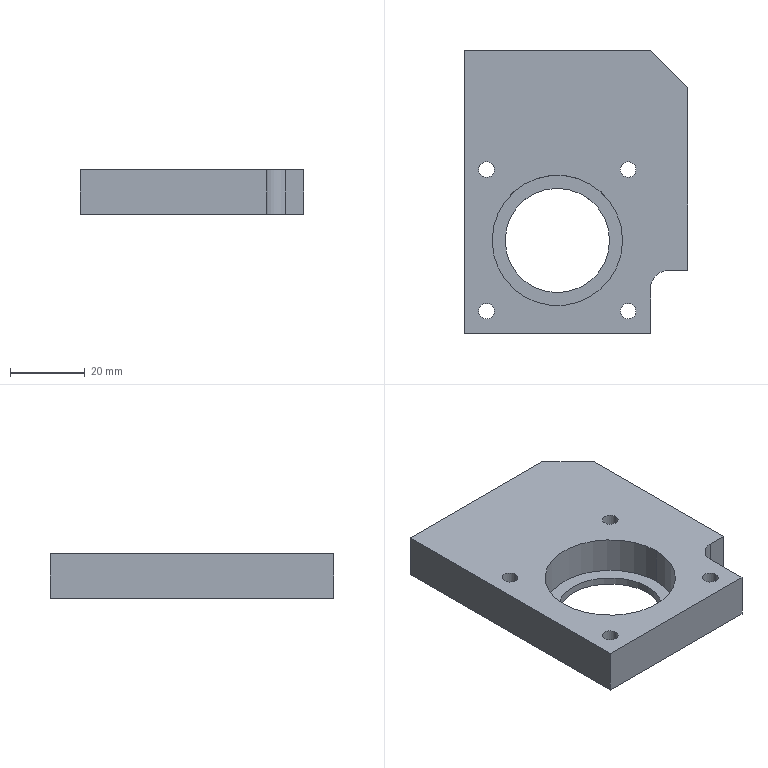Part | SolidWorks | features HoleWzd 2, MoveFace 2, MirrorStock 1 | 1 solid | 43 faces | box 60 x 76 x 12 mm | volume 39739 mm3 | cylinder 23 | cone 10 | plane 10 | commonest cylinder face diameters 4.2 x18 28 x2 35 x2 10 x1
STEP:
#1=CARTESIAN_POINT('',(17.6,22.,2.1));
#2=VERTEX_POINT('',#1);
#3=CARTESIAN_POINT('',(17.6,22.,-2.1));
#4=VERTEX_POINT('',#3);
#5=CARTESIAN_POINT('',(17.6,22.,0.));
#6=DIRECTION('',(-1.,0.,0.));
#7=DIRECTION('',(0.,0.,1.));
#8=AXIS2_PLACEMENT_3D('',#5,#6,#7);
#9=CIRCLE('',#8,2.1);
#10=EDGE_CURVE('',#2,#4,#9,.T.);
#11=ORIENTED_EDGE('',*,*,#10,.T.);
#12=CARTESIAN_POINT('',(30.,22.,-2.1));
#13=VERTEX_POINT('',#12);
#14=CARTESIAN_POINT('',(30.,22.,-2.1));
#15=DIRECTION('',(1.,0.,0.));
#16=VECTOR('',#15,1000.);
#17=LINE('',#14,#16);
#18=EDGE_CURVE('',#4,#13,#17,.T.);
#19=ORIENTED_EDGE('',*,*,#18,.T.);
#20=CARTESIAN_POINT('',(30.,22.,2.1));
#21=VERTEX_POINT('',#20);
#22=CARTESIAN_POINT('',(30.,22.,0.));
#23=DIRECTION('',(-1.,0.,0.));
#24=DIRECTION('',(0.,0.,1.));
#25=AXIS2_PLACEMENT_3D('',#22,#23,#24);
#26=CIRCLE('',#25,2.1);
#27=EDGE_CURVE('',#21,#13,#26,.T.);
#28=ORIENTED_EDGE('',*,*,#27,.F.);
#29=CARTESIAN_POINT('',(30.,22.,2.1));
#30=DIRECTION('',(1.,0.,0.));
#31=VECTOR('',#30,1000.);
#32=LINE('',#29,#31);
#33=EDGE_CURVE('',#2,#21,#32,.T.);
#34=ORIENTED_EDGE('',*,*,#33,.F.);
#35=EDGE_LOOP('',(#11,#19,#28,#34));
#36=FACE_OUTER_BOUND('',#35,.T.);
#37=CARTESIAN_POINT('',(30.,22.,0.));
#38=DIRECTION('',(1.,0.,0.));
#39=DIRECTION('',(0.,0.,1.));
#40=AXIS2_PLACEMENT_3D('',#37,#38,#39);
#41=CYLINDRICAL_SURFACE('',#40,2.1);
#42=ADVANCED_FACE('',(#36),#41,.F.);
#43=CARTESIAN_POINT('',(16.338,22.,0.));
#44=VERTEX_POINT('',#43);
#45=CARTESIAN_POINT('',(17.6,22.,2.1));
#46=DIRECTION('',(0.515,0.,0.8572));
#47=VECTOR('',#46,1000.);
#48=LINE('',#45,#47);
#49=EDGE_CURVE('',#44,#2,#48,.T.);
#50=ORIENTED_EDGE('',*,*,#49,.F.);
#51=CARTESIAN_POINT('',(17.6,22.,-2.1));
#52=DIRECTION('',(0.515,0.,-0.8572));
#53=VECTOR('',#52,1000.);
#54=LINE('',#51,#53);
#55=EDGE_CURVE('',#44,#4,#54,.T.);
#56=ORIENTED_EDGE('',*,*,#55,.T.);
#57=ORIENTED_EDGE('',*,*,#10,.F.);
#58=EDGE_LOOP('',(#50,#56,#57));
#59=FACE_OUTER_BOUND('',#58,.T.);
#60=CARTESIAN_POINT('',(17.6,22.,0.));
#61=DIRECTION('',(1.,0.,0.));
#62=DIRECTION('',(0.,0.,1.));
#63=AXIS2_PLACEMENT_3D('',#60,#61,#62);
#64=CONICAL_SURFACE('',#63,2.1,1.03);
#65=ADVANCED_FACE('',(#59),#64,.F.);
#66=CARTESIAN_POINT('',(17.6,-6.,2.1));
#67=VERTEX_POINT('',#66);
#68=CARTESIAN_POINT('',(17.6,-6.,-2.1));
#69=VERTEX_POINT('',#68);
#70=CARTESIAN_POINT('',(17.6,-6.,0.));
#71=DIRECTION('',(-1.,0.,0.));
#72=DIRECTION('',(0.,0.,1.));
#73=AXIS2_PLACEMENT_3D('',#70,#71,#72);
#74=CIRCLE('',#73,2.1);
#75=EDGE_CURVE('',#67,#69,#74,.T.);
#76=ORIENTED_EDGE('',*,*,#75,.T.);
#77=CARTESIAN_POINT('',(30.,-6.,-2.1));
#78=VERTEX_POINT('',#77);
#79=CARTESIAN_POINT('',(30.,-6.,-2.1));
#80=DIRECTION('',(1.,0.,0.));
#81=VECTOR('',#80,1000.);
#82=LINE('',#79,#81);
#83=EDGE_CURVE('',#69,#78,#82,.T.);
#84=ORIENTED_EDGE('',*,*,#83,.T.);
#85=CARTESIAN_POINT('',(30.,-6.,2.1));
#86=VERTEX_POINT('',#85);
#87=CARTESIAN_POINT('',(30.,-6.,0.));
#88=DIRECTION('',(-1.,0.,0.));
#89=DIRECTION('',(0.,0.,1.));
#90=AXIS2_PLACEMENT_3D('',#87,#88,#89);
#91=CIRCLE('',#90,2.1);
#92=EDGE_CURVE('',#86,#78,#91,.T.);
#93=ORIENTED_EDGE('',*,*,#92,.F.);
#94=CARTESIAN_POINT('',(30.,-6.,2.1));
#95=DIRECTION('',(1.,0.,0.));
#96=VECTOR('',#95,1000.);
#97=LINE('',#94,#96);
#98=EDGE_CURVE('',#67,#86,#97,.T.);
#99=ORIENTED_EDGE('',*,*,#98,.F.);
#100=EDGE_LOOP('',(#76,#84,#93,#99));
#101=FACE_OUTER_BOUND('',#100,.T.);
#102=CARTESIAN_POINT('',(30.,-6.,0.));
#103=DIRECTION('',(1.,0.,0.));
#104=DIRECTION('',(0.,0.,1.));
#105=AXIS2_PLACEMENT_3D('',#102,#103,#104);
#106=CYLINDRICAL_SURFACE('',#105,2.1);
#107=ADVANCED_FACE('',(#101),#106,.F.);
#108=CARTESIAN_POINT('',(16.338,-6.,0.));
#109=VERTEX_POINT('',#108);
#110=CARTESIAN_POINT('',(17.6,-6.,2.1));
#111=DIRECTION('',(0.515,0.,0.8572));
#112=VECTOR('',#111,1000.);
#113=LINE('',#110,#112);
#114=EDGE_CURVE('',#109,#67,#113,.T.);
#115=ORIENTED_EDGE('',*,*,#114,.F.);
#116=CARTESIAN_POINT('',(17.6,-6.,-2.1));
#117=DIRECTION('',(0.515,0.,-0.8572));
#118=VECTOR('',#117,1000.);
#119=LINE('',#116,#118);
#120=EDGE_CURVE('',#109,#69,#119,.T.);
#121=ORIENTED_EDGE('',*,*,#120,.T.);
#122=ORIENTED_EDGE('',*,*,#75,.F.);
#123=EDGE_LOOP('',(#115,#121,#122));
#124=FACE_OUTER_BOUND('',#123,.T.);
#125=CARTESIAN_POINT('',(17.6,-6.,0.));
#126=DIRECTION('',(1.,0.,0.));
#127=DIRECTION('',(0.,0.,1.));
#128=AXIS2_PLACEMENT_3D('',#125,#126,#127);
#129=CONICAL_SURFACE('',#128,2.1,1.03);
#130=ADVANCED_FACE('',(#124),#129,.F.);
#131=CARTESIAN_POINT('',(-24.,27.6,-2.1));
#132=VERTEX_POINT('',#131);
#133=CARTESIAN_POINT('',(-24.,27.6,2.1));
#134=VERTEX_POINT('',#133);
#135=CARTESIAN_POINT('',(-24.,27.6,0.));
#136=DIRECTION('',(0.,-1.,0.));
#137=DIRECTION('',(0.,0.,-1.));
#138=AXIS2_PLACEMENT_3D('',#135,#136,#137);
#139=CIRCLE('',#138,2.1);
#140=EDGE_CURVE('',#132,#134,#139,.T.);
#141=ORIENTED_EDGE('',*,*,#140,.T.);
#142=CARTESIAN_POINT('',(-24.,40.,2.1));
#143=VERTEX_POINT('',#142);
#144=CARTESIAN_POINT('',(-24.,40.,2.1));
#145=DIRECTION('',(0.,1.,0.));
#146=VECTOR('',#145,1000.);
#147=LINE('',#144,#146);
#148=EDGE_CURVE('',#134,#143,#147,.T.);
#149=ORIENTED_EDGE('',*,*,#148,.T.);
#150=CARTESIAN_POINT('',(-24.,40.,-2.1));
#151=VERTEX_POINT('',#150);
#152=CARTESIAN_POINT('',(-24.,40.,0.));
#153=DIRECTION('',(0.,-1.,0.));
#154=DIRECTION('',(0.,0.,-1.));
#155=AXIS2_PLACEMENT_3D('',#152,#153,#154);
#156=CIRCLE('',#155,2.1);
#157=EDGE_CURVE('',#151,#143,#156,.T.);
#158=ORIENTED_EDGE('',*,*,#157,.F.);
#159=CARTESIAN_POINT('',(-24.,40.,-2.1));
#160=DIRECTION('',(0.,1.,0.));
#161=VECTOR('',#160,1000.);
#162=LINE('',#159,#161);
#163=EDGE_CURVE('',#132,#151,#162,.T.);
#164=ORIENTED_EDGE('',*,*,#163,.F.);
#165=EDGE_LOOP('',(#141,#149,#158,#164));
#166=FACE_OUTER_BOUND('',#165,.T.);
#167=CARTESIAN_POINT('',(-24.,40.,0.));
#168=DIRECTION('',(0.,1.,0.));
#169=DIRECTION('',(0.,0.,-1.));
#170=AXIS2_PLACEMENT_3D('',#167,#168,#169);
#171=CYLINDRICAL_SURFACE('',#170,2.1);
#172=ADVANCED_FACE('',(#166),#171,.F.);
#173=CARTESIAN_POINT('',(-24.,26.338,0.));
#174=VERTEX_POINT('',#173);
#175=CARTESIAN_POINT('',(-24.,27.6,-2.1));
#176=DIRECTION('',(0.,0.515,-0.8572));
#177=VECTOR('',#176,1000.);
#178=LINE('',#175,#177);
#179=EDGE_CURVE('',#174,#132,#178,.T.);
#180=ORIENTED_EDGE('',*,*,#179,.F.);
#181=CARTESIAN_POINT('',(-24.,27.6,2.1));
#182=DIRECTION('',(0.,0.515,0.8572));
#183=VECTOR('',#182,1000.);
#184=LINE('',#181,#183);
#185=EDGE_CURVE('',#174,#134,#184,.T.);
#186=ORIENTED_EDGE('',*,*,#185,.T.);
#187=ORIENTED_EDGE('',*,*,#140,.F.);
#188=EDGE_LOOP('',(#180,#186,#187));
#189=FACE_OUTER_BOUND('',#188,.T.);
#190=CARTESIAN_POINT('',(-24.,27.6,0.));
#191=DIRECTION('',(0.,1.,0.));
#192=DIRECTION('',(0.,0.,-1.));
#193=AXIS2_PLACEMENT_3D('',#190,#191,#192);
#194=CONICAL_SURFACE('',#193,2.1,1.03);
#195=ADVANCED_FACE('',(#189),#194,.F.);
#196=CARTESIAN_POINT('',(-2.9,27.6,-2.1));
#197=VERTEX_POINT('',#196);
#198=CARTESIAN_POINT('',(-2.9,27.6,2.1));
#199=VERTEX_POINT('',#198);
#200=CARTESIAN_POINT('',(-2.9,27.6,0.));
#201=DIRECTION('',(0.,-1.,0.));
#202=DIRECTION('',(0.,0.,-1.));
#203=AXIS2_PLACEMENT_3D('',#200,#201,#202);
#204=CIRCLE('',#203,2.1);
#205=EDGE_CURVE('',#197,#199,#204,.T.);
#206=ORIENTED_EDGE('',*,*,#205,.T.);
#207=CARTESIAN_POINT('',(-2.9,40.,2.1));
#208=VERTEX_POINT('',#207);
#209=CARTESIAN_POINT('',(-2.9,40.,2.1));
#210=DIRECTION('',(0.,1.,0.));
#211=VECTOR('',#210,1000.);
#212=LINE('',#209,#211);
#213=EDGE_CURVE('',#199,#208,#212,.T.);
#214=ORIENTED_EDGE('',*,*,#213,.T.);
#215=CARTESIAN_POINT('',(-2.9,40.,-2.1));
#216=VERTEX_POINT('',#215);
#217=CARTESIAN_POINT('',(-2.9,40.,0.));
#218=DIRECTION('',(0.,-1.,0.));
#219=DIRECTION('',(0.,0.,-1.));
#220=AXIS2_PLACEMENT_3D('',#217,#218,#219);
#221=CIRCLE('',#220,2.1);
#222=EDGE_CURVE('',#216,#208,#221,.T.);
#223=ORIENTED_EDGE('',*,*,#222,.F.);
#224=CARTESIAN_POINT('',(-2.9,40.,-2.1));
#225=DIRECTION('',(0.,1.,0.));
#226=VECTOR('',#225,1000.);
#227=LINE('',#224,#226);
#228=EDGE_CURVE('',#197,#216,#227,.T.);
#229=ORIENTED_EDGE('',*,*,#228,.F.);
#230=EDGE_LOOP('',(#206,#214,#223,#229));
#231=FACE_OUTER_BOUND('',#230,.T.);
#232=CARTESIAN_POINT('',(-2.9,40.,0.));
#233=DIRECTION('',(0.,1.,0.));
#234=DIRECTION('',(0.,0.,-1.));
#235=AXIS2_PLACEMENT_3D('',#232,#233,#234);
#236=CYLINDRICAL_SURFACE('',#235,2.1);
#237=ADVANCED_FACE('',(#231),#236,.F.);
#238=CARTESIAN_POINT('',(-2.9,26.338,0.));
#239=VERTEX_POINT('',#238);
#240=CARTESIAN_POINT('',(-2.9,27.6,-2.1));
#241=DIRECTION('',(0.,0.515,-0.8572));
#242=VECTOR('',#241,1000.);
#243=LINE('',#240,#242);
#244=EDGE_CURVE('',#239,#197,#243,.T.);
#245=ORIENTED_EDGE('',*,*,#244,.F.);
#246=CARTESIAN_POINT('',(-2.9,27.6,2.1));
#247=DIRECTION('',(0.,0.515,0.8572));
#248=VECTOR('',#247,1000.);
#249=LINE('',#246,#248);
#250=EDGE_CURVE('',#239,#199,#249,.T.);
#251=ORIENTED_EDGE('',*,*,#250,.T.);
#252=ORIENTED_EDGE('',*,*,#205,.F.);
#253=EDGE_LOOP('',(#245,#251,#252));
#254=FACE_OUTER_BOUND('',#253,.T.);
#255=CARTESIAN_POINT('',(-2.9,27.6,0.));
#256=DIRECTION('',(0.,1.,0.));
#257=DIRECTION('',(0.,0.,-1.));
#258=AXIS2_PLACEMENT_3D('',#255,#256,#257);
#259=CONICAL_SURFACE('',#258,2.1,1.03);
#260=ADVANCED_FACE('',(#254),#259,.F.);
#261=CARTESIAN_POINT('',(15.,27.6,-2.1));
#262=VERTEX_POINT('',#261);
#263=CARTESIAN_POINT('',(15.,27.6,2.1));
#264=VERTEX_POINT('',#263);
#265=CARTESIAN_POINT('',(15.,27.6,0.));
#266=DIRECTION('',(0.,-1.,0.));
#267=DIRECTION('',(0.,0.,-1.));
#268=AXIS2_PLACEMENT_3D('',#265,#266,#267);
#269=CIRCLE('',#268,2.1);
#270=EDGE_CURVE('',#262,#264,#269,.T.);
#271=ORIENTED_EDGE('',*,*,#270,.T.);
#272=CARTESIAN_POINT('',(15.,40.,2.1));
#273=VERTEX_POINT('',#272);
#274=CARTESIAN_POINT('',(15.,40.,2.1));
#275=DIRECTION('',(0.,1.,0.));
#276=VECTOR('',#275,1000.);
#277=LINE('',#274,#276);
#278=EDGE_CURVE('',#264,#273,#277,.T.);
#279=ORIENTED_EDGE('',*,*,#278,.T.);
#280=CARTESIAN_POINT('',(15.,40.,-2.1));
#281=VERTEX_POINT('',#280);
#282=CARTESIAN_POINT('',(15.,40.,0.));
#283=DIRECTION('',(0.,-1.,0.));
#284=DIRECTION('',(0.,0.,-1.));
#285=AXIS2_PLACEMENT_3D('',#282,#283,#284);
#286=CIRCLE('',#285,2.1);
#287=EDGE_CURVE('',#281,#273,#286,.T.);
#288=ORIENTED_EDGE('',*,*,#287,.F.);
#289=CARTESIAN_POINT('',(15.,40.,-2.1));
#290=DIRECTION('',(0.,1.,0.));
#291=VECTOR('',#290,1000.);
#292=LINE('',#289,#291);
#293=EDGE_CURVE('',#262,#281,#292,.T.);
#294=ORIENTED_EDGE('',*,*,#293,.F.);
#295=EDGE_LOOP('',(#271,#279,#288,#294));
#296=FACE_OUTER_BOUND('',#295,.T.);
#297=CARTESIAN_POINT('',(15.,40.,0.));
#298=DIRECTION('',(0.,1.,0.));
#299=DIRECTION('',(0.,0.,-1.));
#300=AXIS2_PLACEMENT_3D('',#297,#298,#299);
#301=CYLINDRICAL_SURFACE('',#300,2.1);
#302=ADVANCED_FACE('',(#296),#301,.F.);
#303=CARTESIAN_POINT('',(15.,26.338,0.));
#304=VERTEX_POINT('',#303);
#305=CARTESIAN_POINT('',(15.,27.6,-2.1));
#306=DIRECTION('',(0.,0.515,-0.8572));
#307=VECTOR('',#306,1000.);
#308=LINE('',#305,#307);
#309=EDGE_CURVE('',#304,#262,#308,.T.);
#310=ORIENTED_EDGE('',*,*,#309,.F.);
#311=CARTESIAN_POINT('',(15.,27.6,2.1));
#312=DIRECTION('',(0.,0.515,0.8572));
#313=VECTOR('',#312,1000.);
#314=LINE('',#311,#313);
#315=EDGE_CURVE('',#304,#264,#314,.T.);
#316=ORIENTED_EDGE('',*,*,#315,.T.);
#317=ORIENTED_EDGE('',*,*,#270,.F.);
#318=EDGE_LOOP('',(#310,#316,#317));
#319=FACE_OUTER_BOUND('',#318,.T.);
#320=CARTESIAN_POINT('',(15.,27.6,0.));
#321=DIRECTION('',(0.,1.,0.));
#322=DIRECTION('',(0.,0.,-1.));
#323=AXIS2_PLACEMENT_3D('',#320,#321,#322);
#324=CONICAL_SURFACE('',#323,2.1,1.03);
#325=ADVANCED_FACE('',(#319),#324,.F.);
#326=CARTESIAN_POINT('',(11.9,8.,-6.));
#327=VERTEX_POINT('',#326);
#328=CARTESIAN_POINT('',(16.1,8.,-6.));
#329=VERTEX_POINT('',#328);
#330=CARTESIAN_POINT('',(14.,8.,-6.));
#331=DIRECTION('',(0.,0.,-1.));
#332=DIRECTION('',(-1.,0.,0.));
#333=AXIS2_PLACEMENT_3D('',#330,#331,#332);
#334=CIRCLE('',#333,2.1);
#335=EDGE_CURVE('',#327,#329,#334,.T.);
#336=ORIENTED_EDGE('',*,*,#335,.T.);
#337=CARTESIAN_POINT('',(16.1,8.,6.));
#338=VERTEX_POINT('',#337);
#339=CARTESIAN_POINT('',(16.1,8.,6.));
#340=DIRECTION('',(0.,0.,1.));
#341=VECTOR('',#340,1000.);
#342=LINE('',#339,#341);
#343=EDGE_CURVE('',#329,#338,#342,.T.);
#344=ORIENTED_EDGE('',*,*,#343,.T.);
#345=CARTESIAN_POINT('',(11.9,8.,6.));
#346=VERTEX_POINT('',#345);
#347=CARTESIAN_POINT('',(14.,8.,6.));
#348=DIRECTION('',(0.,0.,-1.));
#349=DIRECTION('',(-1.,0.,0.));
#350=AXIS2_PLACEMENT_3D('',#347,#348,#349);
#351=CIRCLE('',#350,2.1);
#352=EDGE_CURVE('',#346,#338,#351,.T.);
#353=ORIENTED_EDGE('',*,*,#352,.F.);
#354=CARTESIAN_POINT('',(11.9,8.,6.));
#355=DIRECTION('',(0.,0.,1.));
#356=VECTOR('',#355,1000.);
#357=LINE('',#354,#356);
#358=EDGE_CURVE('',#327,#346,#357,.T.);
#359=ORIENTED_EDGE('',*,*,#358,.F.);
#360=EDGE_LOOP('',(#336,#344,#353,#359));
#361=FACE_OUTER_BOUND('',#360,.T.);
#362=CARTESIAN_POINT('',(14.,8.,6.));
#363=DIRECTION('',(0.,0.,1.));
#364=DIRECTION('',(-1.,0.,0.));
#365=AXIS2_PLACEMENT_3D('',#362,#363,#364);
#366=CYLINDRICAL_SURFACE('',#365,2.1);
#367=ADVANCED_FACE('',(#361),#366,.F.);
#368=CARTESIAN_POINT('',(11.9,-30.,-6.));
#369=VERTEX_POINT('',#368);
#370=CARTESIAN_POINT('',(16.1,-30.,-6.));
#371=VERTEX_POINT('',#370);
#372=CARTESIAN_POINT('',(14.,-30.,-6.));
#373=DIRECTION('',(0.,0.,-1.));
#374=DIRECTION('',(-1.,0.,0.));
#375=AXIS2_PLACEMENT_3D('',#372,#373,#374);
#376=CIRCLE('',#375,2.1);
#377=EDGE_CURVE('',#369,#371,#376,.T.);
#378=ORIENTED_EDGE('',*,*,#377,.T.);
#379=CARTESIAN_POINT('',(16.1,-30.,6.));
#380=VERTEX_POINT('',#379);
#381=CARTESIAN_POINT('',(16.1,-30.,6.));
#382=DIRECTION('',(0.,0.,1.));
#383=VECTOR('',#382,1000.);
#384=LINE('',#381,#383);
#385=EDGE_CURVE('',#371,#380,#384,.T.);
#386=ORIENTED_EDGE('',*,*,#385,.T.);
#387=CARTESIAN_POINT('',(11.9,-30.,6.));
#388=VERTEX_POINT('',#387);
#389=CARTESIAN_POINT('',(14.,-30.,6.));
#390=DIRECTION('',(0.,0.,-1.));
#391=DIRECTION('',(-1.,0.,0.));
#392=AXIS2_PLACEMENT_3D('',#389,#390,#391);
#393=CIRCLE('',#392,2.1);
#394=EDGE_CURVE('',#388,#380,#393,.T.);
#395=ORIENTED_EDGE('',*,*,#394,.F.);
#396=CARTESIAN_POINT('',(11.9,-30.,6.));
#397=DIRECTION('',(0.,0.,1.));
#398=VECTOR('',#397,1000.);
#399=LINE('',#396,#398);
#400=EDGE_CURVE('',#369,#388,#399,.T.);
#401=ORIENTED_EDGE('',*,*,#400,.F.);
#402=EDGE_LOOP('',(#378,#386,#395,#401));
#403=FACE_OUTER_BOUND('',#402,.T.);
#404=CARTESIAN_POINT('',(14.,-30.,6.));
#405=DIRECTION('',(0.,0.,1.));
#406=DIRECTION('',(-1.,0.,0.));
#407=AXIS2_PLACEMENT_3D('',#404,#405,#406);
#408=CYLINDRICAL_SURFACE('',#407,2.1);
#409=ADVANCED_FACE('',(#403),#408,.F.);
#410=CARTESIAN_POINT('',(-26.1,-30.,-6.));
#411=VERTEX_POINT('',#410);
#412=CARTESIAN_POINT('',(-21.9,-30.,-6.));
#413=VERTEX_POINT('',#412);
#414=CARTESIAN_POINT('',(-24.,-30.,-6.));
#415=DIRECTION('',(0.,0.,-1.));
#416=DIRECTION('',(-1.,0.,0.));
#417=AXIS2_PLACEMENT_3D('',#414,#415,#416);
#418=CIRCLE('',#417,2.1);
#419=EDGE_CURVE('',#411,#413,#418,.T.);
#420=ORIENTED_EDGE('',*,*,#419,.T.);
#421=CARTESIAN_POINT('',(-21.9,-30.,6.));
#422=VERTEX_POINT('',#421);
#423=CARTESIAN_POINT('',(-21.9,-30.,6.));
#424=DIRECTION('',(0.,0.,1.));
#425=VECTOR('',#424,1000.);
#426=LINE('',#423,#425);
#427=EDGE_CURVE('',#413,#422,#426,.T.);
#428=ORIENTED_EDGE('',*,*,#427,.T.);
#429=CARTESIAN_POINT('',(-26.1,-30.,6.));
#430=VERTEX_POINT('',#429);
#431=CARTESIAN_POINT('',(-24.,-30.,6.));
#432=DIRECTION('',(0.,0.,-1.));
#433=DIRECTION('',(-1.,0.,0.));
#434=AXIS2_PLACEMENT_3D('',#431,#432,#433);
#435=CIRCLE('',#434,2.1);
#436=EDGE_CURVE('',#430,#422,#435,.T.);
#437=ORIENTED_EDGE('',*,*,#436,.F.);
#438=CARTESIAN_POINT('',(-26.1,-30.,6.));
#439=DIRECTION('',(0.,0.,1.));
#440=VECTOR('',#439,1000.);
#441=LINE('',#438,#440);
#442=EDGE_CURVE('',#411,#430,#441,.T.);
#443=ORIENTED_EDGE('',*,*,#442,.F.);
#444=EDGE_LOOP('',(#420,#428,#437,#443));
#445=FACE_OUTER_BOUND('',#444,.T.);
#446=CARTESIAN_POINT('',(-24.,-30.,6.));
#447=DIRECTION('',(0.,0.,1.));
#448=DIRECTION('',(-1.,0.,0.));
#449=AXIS2_PLACEMENT_3D('',#446,#447,#448);
#450=CYLINDRICAL_SURFACE('',#449,2.1);
#451=ADVANCED_FACE('',(#445),#450,.F.);
#452=CARTESIAN_POINT('',(-26.1,8.,-6.));
#453=VERTEX_POINT('',#452);
#454=CARTESIAN_POINT('',(-21.9,8.,-6.));
#455=VERTEX_POINT('',#454);
#456=CARTESIAN_POINT('',(-24.,8.,-6.));
#457=DIRECTION('',(0.,0.,-1.));
#458=DIRECTION('',(-1.,0.,0.));
#459=AXIS2_PLACEMENT_3D('',#456,#457,#458);
#460=CIRCLE('',#459,2.1);
#461=EDGE_CURVE('',#453,#455,#460,.T.);
#462=ORIENTED_EDGE('',*,*,#461,.T.);
#463=CARTESIAN_POINT('',(-21.9,8.,6.));
#464=VERTEX_POINT('',#463);
#465=CARTESIAN_POINT('',(-21.9,8.,6.));
#466=DIRECTION('',(0.,0.,1.));
#467=VECTOR('',#466,1000.);
#468=LINE('',#465,#467);
#469=EDGE_CURVE('',#455,#464,#468,.T.);
#470=ORIENTED_EDGE('',*,*,#469,.T.);
#471=CARTESIAN_POINT('',(-26.1,8.,6.));
#472=VERTEX_POINT('',#471);
#473=CARTESIAN_POINT('',(-24.,8.,6.));
#474=DIRECTION('',(0.,0.,-1.));
#475=DIRECTION('',(-1.,0.,0.));
#476=AXIS2_PLACEMENT_3D('',#473,#474,#475);
#477=CIRCLE('',#476,2.1);
#478=EDGE_CURVE('',#472,#464,#477,.T.);
#479=ORIENTED_EDGE('',*,*,#478,.F.);
#480=CARTESIAN_POINT('',(-26.1,8.,6.));
#481=DIRECTION('',(0.,0.,1.));
#482=VECTOR('',#481,1000.);
#483=LINE('',#480,#482);
#484=EDGE_CURVE('',#453,#472,#483,.T.);
#485=ORIENTED_EDGE('',*,*,#484,.F.);
#486=EDGE_LOOP('',(#462,#470,#479,#485));
#487=FACE_OUTER_BOUND('',#486,.T.);
#488=CARTESIAN_POINT('',(-24.,8.,6.));
#489=DIRECTION('',(0.,0.,1.));
#490=DIRECTION('',(-1.,0.,0.));
#491=AXIS2_PLACEMENT_3D('',#488,#489,#490);
#492=CYLINDRICAL_SURFACE('',#491,2.1);
#493=ADVANCED_FACE('',(#487),#492,.F.);
#494=CARTESIAN_POINT('',(-19.,-11.,-6.));
#495=VERTEX_POINT('',#494);
#496=CARTESIAN_POINT('',(9.,-11.,-6.));
#497=VERTEX_POINT('',#496);
#498=CARTESIAN_POINT('',(-5.,-11.,-6.));
#499=DIRECTION('',(0.,0.,-1.));
#500=DIRECTION('',(-1.,0.,0.));
#501=AXIS2_PLACEMENT_3D('',#498,#499,#500);
#502=CIRCLE('',#501,14.);
#503=EDGE_CURVE('',#495,#497,#502,.T.);
#504=ORIENTED_EDGE('',*,*,#503,.T.);
#505=CARTESIAN_POINT('',(9.,-11.,-4.));
#506=VERTEX_POINT('',#505);
#507=CARTESIAN_POINT('',(9.,-11.,-6.));
#508=DIRECTION('',(0.,0.,1.));
#509=VECTOR('',#508,1000.);
#510=LINE('',#507,#509);
#511=EDGE_CURVE('',#497,#506,#510,.T.);
#512=ORIENTED_EDGE('',*,*,#511,.T.);
#513=CARTESIAN_POINT('',(-19.,-11.,-4.));
#514=VERTEX_POINT('',#513);
#515=CARTESIAN_POINT('',(-5.,-11.,-4.));
#516=DIRECTION('',(0.,0.,-1.));
#517=DIRECTION('',(-1.,0.,0.));
#518=AXIS2_PLACEMENT_3D('',#515,#516,#517);
#519=CIRCLE('',#518,14.);
#520=EDGE_CURVE('',#514,#506,#519,.T.);
#521=ORIENTED_EDGE('',*,*,#520,.F.);
#522=CARTESIAN_POINT('',(-19.,-11.,-6.));
#523=DIRECTION('',(0.,0.,1.));
#524=VECTOR('',#523,1000.);
#525=LINE('',#522,#524);
#526=EDGE_CURVE('',#495,#514,#525,.T.);
#527=ORIENTED_EDGE('',*,*,#526,.F.);
#528=EDGE_LOOP('',(#504,#512,#521,#527));
#529=FACE_OUTER_BOUND('',#528,.T.);
#530=CARTESIAN_POINT('',(-5.,-11.,-6.));
#531=DIRECTION('',(0.,0.,1.));
#532=DIRECTION('',(-1.,0.,0.));
#533=AXIS2_PLACEMENT_3D('',#530,#531,#532);
#534=CYLINDRICAL_SURFACE('',#533,14.);
#535=ADVANCED_FACE('',(#529),#534,.F.);
#536=CARTESIAN_POINT('',(12.5,-11.,-4.));
#537=VERTEX_POINT('',#536);
#538=CARTESIAN_POINT('',(-22.5,-11.,-4.));
#539=VERTEX_POINT('',#538);
#540=CARTESIAN_POINT('',(-5.,-11.,-4.));
#541=DIRECTION('',(0.,0.,1.));
#542=DIRECTION('',(1.,0.,0.));
#543=AXIS2_PLACEMENT_3D('',#540,#541,#542);
#544=CIRCLE('',#543,17.5);
#545=EDGE_CURVE('',#537,#539,#544,.T.);
#546=ORIENTED_EDGE('',*,*,#545,.F.);
#547=CARTESIAN_POINT('',(12.5,-11.,6.));
#548=VERTEX_POINT('',#547);
#549=CARTESIAN_POINT('',(12.5,-11.,-4.));
#550=DIRECTION('',(0.,0.,1.));
#551=VECTOR('',#550,1000.);
#552=LINE('',#549,#551);
#553=EDGE_CURVE('',#537,#548,#552,.T.);
#554=ORIENTED_EDGE('',*,*,#553,.T.);
#555=CARTESIAN_POINT('',(-22.5,-11.,6.));
#556=VERTEX_POINT('',#555);
#557=CARTESIAN_POINT('',(-5.,-11.,6.));
#558=DIRECTION('',(0.,0.,1.));
#559=DIRECTION('',(1.,0.,0.));
#560=AXIS2_PLACEMENT_3D('',#557,#558,#559);
#561=CIRCLE('',#560,17.5);
#562=EDGE_CURVE('',#548,#556,#561,.T.);
#563=ORIENTED_EDGE('',*,*,#562,.T.);
#564=CARTESIAN_POINT('',(-22.5,-11.,-4.));
#565=DIRECTION('',(0.,0.,1.));
#566=VECTOR('',#565,1000.);
#567=LINE('',#564,#566);
#568=EDGE_CURVE('',#539,#556,#567,.T.);
#569=ORIENTED_EDGE('',*,*,#568,.F.);
#570=EDGE_LOOP('',(#546,#554,#563,#569));
#571=FACE_OUTER_BOUND('',#570,.T.);
#572=CARTESIAN_POINT('',(-5.,-11.,-4.));
#573=DIRECTION('',(0.,0.,1.));
#574=DIRECTION('',(-1.,0.,0.));
#575=AXIS2_PLACEMENT_3D('',#572,#573,#574);
#576=CYLINDRICAL_SURFACE('',#575,17.5);
#577=ADVANCED_FACE('',(#571),#576,.F.);
#578=ORIENTED_EDGE('',*,*,#27,.T.);
#579=CARTESIAN_POINT('',(30.,22.,0.));
#580=DIRECTION('',(-1.,0.,0.));
#581=DIRECTION('',(0.,0.,1.));
#582=AXIS2_PLACEMENT_3D('',#579,#580,#581);
#583=CIRCLE('',#582,2.1);
#584=EDGE_CURVE('',#13,#21,#583,.T.);
#585=ORIENTED_EDGE('',*,*,#584,.T.);
#586=EDGE_LOOP('',(#578,#585));
#587=FACE_BOUND('',#586,.T.);
#588=ORIENTED_EDGE('',*,*,#92,.T.);
#589=CARTESIAN_POINT('',(30.,-6.,0.));
#590=DIRECTION('',(-1.,0.,0.));
#591=DIRECTION('',(0.,0.,1.));
#592=AXIS2_PLACEMENT_3D('',#589,#590,#591);
#593=CIRCLE('',#592,2.1);
#594=EDGE_CURVE('',#78,#86,#593,.T.);
#595=ORIENTED_EDGE('',*,*,#594,.T.);
#596=EDGE_LOOP('',(#588,#595));
#597=FACE_BOUND('',#596,.T.);
#598=CARTESIAN_POINT('',(30.,-19.,6.));
#599=VERTEX_POINT('',#598);
#600=CARTESIAN_POINT('',(30.,30.,6.));
#601=VERTEX_POINT('',#600);
#602=CARTESIAN_POINT('',(30.,-41.,6.));
#603=DIRECTION('',(0.,1.,0.));
#604=VECTOR('',#603,1000.);
#605=LINE('',#602,#604);
#606=EDGE_CURVE('',#599,#601,#605,.T.);
#607=ORIENTED_EDGE('',*,*,#606,.F.);
#608=CARTESIAN_POINT('',(30.,-19.,-6.));
#609=VERTEX_POINT('',#608);
#610=CARTESIAN_POINT('',(30.,-19.,6.));
#611=DIRECTION('',(0.,0.,-1.));
#612=VECTOR('',#611,1000.);
#613=LINE('',#610,#612);
#614=EDGE_CURVE('',#599,#609,#613,.T.);
#615=ORIENTED_EDGE('',*,*,#614,.T.);
#616=CARTESIAN_POINT('',(30.,30.,-6.));
#617=VERTEX_POINT('',#616);
#618=CARTESIAN_POINT('',(30.,-41.,-6.));
#619=DIRECTION('',(0.,1.,0.));
#620=VECTOR('',#619,1000.);
#621=LINE('',#618,#620);
#622=EDGE_CURVE('',#609,#617,#621,.T.);
#623=ORIENTED_EDGE('',*,*,#622,.T.);
#624=CARTESIAN_POINT('',(30.,30.,-6.));
#625=DIRECTION('',(0.,0.,-1.));
#626=VECTOR('',#625,1000.);
#627=LINE('',#624,#626);
#628=EDGE_CURVE('',#601,#617,#627,.T.);
#629=ORIENTED_EDGE('',*,*,#628,.F.);
#630=EDGE_LOOP('',(#607,#615,#623,#629));
#631=FACE_OUTER_BOUND('',#630,.T.);
#632=CARTESIAN_POINT('',(30.,-41.,-6.));
#633=DIRECTION('',(-1.,0.,0.));
#634=DIRECTION('',(0.,0.,-1.));
#635=AXIS2_PLACEMENT_3D('',#632,#633,#634);
#636=PLANE('',#635);
#637=ADVANCED_FACE('',(#587,#597,#631),#636,.F.);
#638=ORIENTED_EDGE('',*,*,#157,.T.);
#639=CARTESIAN_POINT('',(-24.,40.,0.));
#640=DIRECTION('',(0.,-1.,0.));
#641=DIRECTION('',(0.,0.,-1.));
#642=AXIS2_PLACEMENT_3D('',#639,#640,#641);
#643=CIRCLE('',#642,2.1);
#644=EDGE_CURVE('',#143,#151,#643,.T.);
#645=ORIENTED_EDGE('',*,*,#644,.T.);
#646=EDGE_LOOP('',(#638,#645));
#647=FACE_BOUND('',#646,.T.);
#648=ORIENTED_EDGE('',*,*,#222,.T.);
#649=CARTESIAN_POINT('',(-2.9,40.,0.));
#650=DIRECTION('',(0.,-1.,0.));
#651=DIRECTION('',(0.,0.,-1.));
#652=AXIS2_PLACEMENT_3D('',#649,#650,#651);
#653=CIRCLE('',#652,2.1);
#654=EDGE_CURVE('',#208,#216,#653,.T.);
#655=ORIENTED_EDGE('',*,*,#654,.T.);
#656=EDGE_LOOP('',(#648,#655));
#657=FACE_BOUND('',#656,.T.);
#658=ORIENTED_EDGE('',*,*,#287,.T.);
#659=CARTESIAN_POINT('',(15.,40.,0.));
#660=DIRECTION('',(0.,-1.,0.));
#661=DIRECTION('',(0.,0.,-1.));
#662=AXIS2_PLACEMENT_3D('',#659,#660,#661);
#663=CIRCLE('',#662,2.1);
#664=EDGE_CURVE('',#273,#281,#663,.T.);
#665=ORIENTED_EDGE('',*,*,#664,.T.);
#666=EDGE_LOOP('',(#658,#665));
#667=FACE_BOUND('',#666,.T.);
#668=CARTESIAN_POINT('',(20.,40.,-6.));
#669=VERTEX_POINT('',#668);
#670=CARTESIAN_POINT('',(-30.,40.,-6.));
#671=VERTEX_POINT('',#670);
#672=CARTESIAN_POINT('',(-30.,40.,-6.));
#673=DIRECTION('',(-1.,0.,0.));
#674=VECTOR('',#673,1000.);
#675=LINE('',#672,#674);
#676=EDGE_CURVE('',#669,#671,#675,.T.);
#677=ORIENTED_EDGE('',*,*,#676,.T.);
#678=CARTESIAN_POINT('',(-30.,40.,6.));
#679=VERTEX_POINT('',#678);
#680=CARTESIAN_POINT('',(-30.,40.,-6.));
#681=DIRECTION('',(0.,0.,1.));
#682=VECTOR('',#681,1000.);
#683=LINE('',#680,#682);
#684=EDGE_CURVE('',#671,#679,#683,.T.);
#685=ORIENTED_EDGE('',*,*,#684,.T.);
#686=CARTESIAN_POINT('',(20.,40.,6.));
#687=VERTEX_POINT('',#686);
#688=CARTESIAN_POINT('',(-30.,40.,6.));
#689=DIRECTION('',(-1.,0.,0.));
#690=VECTOR('',#689,1000.);
#691=LINE('',#688,#690);
#692=EDGE_CURVE('',#687,#679,#691,.T.);
#693=ORIENTED_EDGE('',*,*,#692,.F.);
#694=CARTESIAN_POINT('',(20.,40.,-6.));
#695=DIRECTION('',(0.,0.,1.));
#696=VECTOR('',#695,1000.);
#697=LINE('',#694,#696);
#698=EDGE_CURVE('',#669,#687,#697,.T.);
#699=ORIENTED_EDGE('',*,*,#698,.F.);
#700=EDGE_LOOP('',(#677,#685,#693,#699));
#701=FACE_OUTER_BOUND('',#700,.T.);
#702=CARTESIAN_POINT('',(-30.,40.,-6.));
#703=DIRECTION('',(0.,-1.,0.));
#704=DIRECTION('',(0.,0.,1.));
#705=AXIS2_PLACEMENT_3D('',#702,#703,#704);
#706=PLANE('',#705);
#707=ADVANCED_FACE('',(#647,#657,#667,#701),#706,.F.);
#708=CARTESIAN_POINT('',(-30.,-36.,6.));
#709=VERTEX_POINT('',#708);
#710=CARTESIAN_POINT('',(-30.,-41.,6.));
#711=DIRECTION('',(0.,-1.,0.));
#712=VECTOR('',#711,1000.);
#713=LINE('',#710,#712);
#714=EDGE_CURVE('',#679,#709,#713,.T.);
#715=ORIENTED_EDGE('',*,*,#714,.F.);
#716=ORIENTED_EDGE('',*,*,#684,.F.);
#717=CARTESIAN_POINT('',(-30.,-36.,-6.));
#718=VERTEX_POINT('',#717);
#719=CARTESIAN_POINT('',(-30.,-41.,-6.));
#720=DIRECTION('',(0.,-1.,0.));
#721=VECTOR('',#720,1000.);
#722=LINE('',#719,#721);
#723=EDGE_CURVE('',#671,#718,#722,.T.);
#724=ORIENTED_EDGE('',*,*,#723,.T.);
#725=CARTESIAN_POINT('',(-30.,-36.,-6.));
#726=DIRECTION('',(0.,0.,1.));
#727=VECTOR('',#726,1000.);
#728=LINE('',#725,#727);
#729=EDGE_CURVE('',#718,#709,#728,.T.);
#730=ORIENTED_EDGE('',*,*,#729,.T.);
#731=EDGE_LOOP('',(#715,#716,#724,#730));
#732=FACE_OUTER_BOUND('',#731,.T.);
#733=CARTESIAN_POINT('',(-30.,-41.,-6.));
#734=DIRECTION('',(1.,0.,0.));
#735=DIRECTION('',(0.,0.,1.));
#736=AXIS2_PLACEMENT_3D('',#733,#734,#735);
#737=PLANE('',#736);
#738=ADVANCED_FACE('',(#732),#737,.F.);
#739=CARTESIAN_POINT('',(20.,-36.,6.));
#740=VERTEX_POINT('',#739);
#741=CARTESIAN_POINT('',(-30.,-36.,6.));
#742=DIRECTION('',(1.,0.,0.));
#743=VECTOR('',#742,1000.);
#744=LINE('',#741,#743);
#745=EDGE_CURVE('',#709,#740,#744,.T.);
#746=ORIENTED_EDGE('',*,*,#745,.F.);
#747=ORIENTED_EDGE('',*,*,#729,.F.);
#748=CARTESIAN_POINT('',(20.,-36.,-6.));
#749=VERTEX_POINT('',#748);
#750=CARTESIAN_POINT('',(-30.,-36.,-6.));
#751=DIRECTION('',(1.,0.,0.));
#752=VECTOR('',#751,1000.);
#753=LINE('',#750,#752);
#754=EDGE_CURVE('',#718,#749,#753,.T.);
#755=ORIENTED_EDGE('',*,*,#754,.T.);
#756=CARTESIAN_POINT('',(20.,-36.,6.));
#757=DIRECTION('',(0.,0.,-1.));
#758=VECTOR('',#757,1000.);
#759=LINE('',#756,#758);
#760=EDGE_CURVE('',#740,#749,#759,.T.);
#761=ORIENTED_EDGE('',*,*,#760,.F.);
#762=EDGE_LOOP('',(#746,#747,#755,#761));
#763=FACE_OUTER_BOUND('',#762,.T.);
#764=CARTESIAN_POINT('',(-30.,-36.,-6.));
#765=DIRECTION('',(0.,1.,0.));
#766=DIRECTION('',(0.,0.,-1.));
#767=AXIS2_PLACEMENT_3D('',#764,#765,#766);
#768=PLANE('',#767);
#769=ADVANCED_FACE('',(#763),#768,.F.);
#770=ORIENTED_EDGE('',*,*,#335,.F.);
#771=CARTESIAN_POINT('',(14.,8.,-6.));
#772=DIRECTION('',(0.,0.,-1.));
#773=DIRECTION('',(-1.,0.,0.));
#774=AXIS2_PLACEMENT_3D('',#771,#772,#773);
#775=CIRCLE('',#774,2.1);
#776=EDGE_CURVE('',#329,#327,#775,.T.);
#777=ORIENTED_EDGE('',*,*,#776,.F.);
#778=EDGE_LOOP('',(#770,#777));
#779=FACE_BOUND('',#778,.T.);
#780=ORIENTED_EDGE('',*,*,#377,.F.);
#781=CARTESIAN_POINT('',(14.,-30.,-6.));
#782=DIRECTION('',(0.,0.,-1.));
#783=DIRECTION('',(-1.,0.,0.));
#784=AXIS2_PLACEMENT_3D('',#781,#782,#783);
#785=CIRCLE('',#784,2.1);
#786=EDGE_CURVE('',#371,#369,#785,.T.);
#787=ORIENTED_EDGE('',*,*,#786,.F.);
#788=EDGE_LOOP('',(#780,#787));
#789=FACE_BOUND('',#788,.T.);
#790=ORIENTED_EDGE('',*,*,#419,.F.);
#791=CARTESIAN_POINT('',(-24.,-30.,-6.));
#792=DIRECTION('',(0.,0.,-1.));
#793=DIRECTION('',(-1.,0.,0.));
#794=AXIS2_PLACEMENT_3D('',#791,#792,#793);
#795=CIRCLE('',#794,2.1);
#796=EDGE_CURVE('',#413,#411,#795,.T.);
#797=ORIENTED_EDGE('',*,*,#796,.F.);
#798=EDGE_LOOP('',(#790,#797));
#799=FACE_BOUND('',#798,.T.);
#800=ORIENTED_EDGE('',*,*,#461,.F.);
#801=CARTESIAN_POINT('',(-24.,8.,-6.));
#802=DIRECTION('',(0.,0.,-1.));
#803=DIRECTION('',(-1.,0.,0.));
#804=AXIS2_PLACEMENT_3D('',#801,#802,#803);
#805=CIRCLE('',#804,2.1);
#806=EDGE_CURVE('',#455,#453,#805,.T.);
#807=ORIENTED_EDGE('',*,*,#806,.F.);
#808=EDGE_LOOP('',(#800,#807));
#809=FACE_BOUND('',#808,.T.);
#810=ORIENTED_EDGE('',*,*,#503,.F.);
#811=CARTESIAN_POINT('',(-5.,-11.,-6.));
#812=DIRECTION('',(0.,0.,-1.));
#813=DIRECTION('',(-1.,0.,0.));
#814=AXIS2_PLACEMENT_3D('',#811,#812,#813);
#815=CIRCLE('',#814,14.);
#816=EDGE_CURVE('',#497,#495,#815,.T.);
#817=ORIENTED_EDGE('',*,*,#816,.F.);
#818=EDGE_LOOP('',(#810,#817));
#819=FACE_BOUND('',#818,.T.);
#820=ORIENTED_EDGE('',*,*,#622,.F.);
#821=CARTESIAN_POINT('',(25.,-19.,-6.));
#822=VERTEX_POINT('',#821);
#823=CARTESIAN_POINT('',(20.,-19.,-6.));
#824=DIRECTION('',(-1.,0.,0.));
#825=VECTOR('',#824,1000.);
#826=LINE('',#823,#825);
#827=EDGE_CURVE('',#609,#822,#826,.T.);
#828=ORIENTED_EDGE('',*,*,#827,.T.);
#829=CARTESIAN_POINT('',(20.,-24.,-6.));
#830=VERTEX_POINT('',#829);
#831=CARTESIAN_POINT('',(25.,-24.,-6.));
#832=DIRECTION('',(0.,0.,-1.));
#833=DIRECTION('',(-1.,0.,0.));
#834=AXIS2_PLACEMENT_3D('',#831,#832,#833);
#835=CIRCLE('',#834,5.);
#836=EDGE_CURVE('',#830,#822,#835,.T.);
#837=ORIENTED_EDGE('',*,*,#836,.F.);
#838=CARTESIAN_POINT('',(20.,-41.,-6.));
#839=DIRECTION('',(0.,-1.,0.));
#840=VECTOR('',#839,1000.);
#841=LINE('',#838,#840);
#842=EDGE_CURVE('',#830,#749,#841,.T.);
#843=ORIENTED_EDGE('',*,*,#842,.T.);
#844=ORIENTED_EDGE('',*,*,#754,.F.);
#845=ORIENTED_EDGE('',*,*,#723,.F.);
#846=ORIENTED_EDGE('',*,*,#676,.F.);
#847=CARTESIAN_POINT('',(20.,40.,-6.));
#848=DIRECTION('',(-0.7071,0.7071,0.));
#849=VECTOR('',#848,1000.);
#850=LINE('',#847,#849);
#851=EDGE_CURVE('',#617,#669,#850,.T.);
#852=ORIENTED_EDGE('',*,*,#851,.F.);
#853=EDGE_LOOP('',(#820,#828,#837,#843,#844,#845,#846,#852));
#854=FACE_OUTER_BOUND('',#853,.T.);
#855=CARTESIAN_POINT('',(0.,0.,-6.));
#856=DIRECTION('',(0.,0.,1.));
#857=DIRECTION('',(-1.,0.,0.));
#858=AXIS2_PLACEMENT_3D('',#855,#856,#857);
#859=PLANE('',#858);
#860=ADVANCED_FACE('',(#779,#789,#799,#809,#819,#854),#859,.F.);
#861=ORIENTED_EDGE('',*,*,#352,.T.);
#862=CARTESIAN_POINT('',(14.,8.,6.));
#863=DIRECTION('',(0.,0.,-1.));
#864=DIRECTION('',(-1.,0.,0.));
#865=AXIS2_PLACEMENT_3D('',#862,#863,#864);
#866=CIRCLE('',#865,2.1);
#867=EDGE_CURVE('',#338,#346,#866,.T.);
#868=ORIENTED_EDGE('',*,*,#867,.T.);
#869=EDGE_LOOP('',(#861,#868));
#870=FACE_BOUND('',#869,.T.);
#871=ORIENTED_EDGE('',*,*,#394,.T.);
#872=CARTESIAN_POINT('',(14.,-30.,6.));
#873=DIRECTION('',(0.,0.,-1.));
#874=DIRECTION('',(-1.,0.,0.));
#875=AXIS2_PLACEMENT_3D('',#872,#873,#874);
#876=CIRCLE('',#875,2.1);
#877=EDGE_CURVE('',#380,#388,#876,.T.);
#878=ORIENTED_EDGE('',*,*,#877,.T.);
#879=EDGE_LOOP('',(#871,#878));
#880=FACE_BOUND('',#879,.T.);
#881=ORIENTED_EDGE('',*,*,#436,.T.);
#882=CARTESIAN_POINT('',(-24.,-30.,6.));
#883=DIRECTION('',(0.,0.,-1.));
#884=DIRECTION('',(-1.,0.,0.));
#885=AXIS2_PLACEMENT_3D('',#882,#883,#884);
#886=CIRCLE('',#885,2.1);
#887=EDGE_CURVE('',#422,#430,#886,.T.);
#888=ORIENTED_EDGE('',*,*,#887,.T.);
#889=EDGE_LOOP('',(#881,#888));
#890=FACE_BOUND('',#889,.T.);
#891=ORIENTED_EDGE('',*,*,#478,.T.);
#892=CARTESIAN_POINT('',(-24.,8.,6.));
#893=DIRECTION('',(0.,0.,-1.));
#894=DIRECTION('',(-1.,0.,0.));
#895=AXIS2_PLACEMENT_3D('',#892,#893,#894);
#896=CIRCLE('',#895,2.1);
#897=EDGE_CURVE('',#464,#472,#896,.T.);
#898=ORIENTED_EDGE('',*,*,#897,.T.);
#899=EDGE_LOOP('',(#891,#898));
#900=FACE_BOUND('',#899,.T.);
#901=ORIENTED_EDGE('',*,*,#692,.T.);
#902=ORIENTED_EDGE('',*,*,#714,.T.);
#903=ORIENTED_EDGE('',*,*,#745,.T.);
#904=CARTESIAN_POINT('',(20.,-24.,6.));
#905=VERTEX_POINT('',#904);
#906=CARTESIAN_POINT('',(20.,-41.,6.));
#907=DIRECTION('',(0.,-1.,0.));
#908=VECTOR('',#907,1000.);
#909=LINE('',#906,#908);
#910=EDGE_CURVE('',#905,#740,#909,.T.);
#911=ORIENTED_EDGE('',*,*,#910,.F.);
#912=CARTESIAN_POINT('',(25.,-19.,6.));
#913=VERTEX_POINT('',#912);
#914=CARTESIAN_POINT('',(25.,-24.,6.));
#915=DIRECTION('',(0.,0.,1.));
#916=DIRECTION('',(-1.,0.,0.));
#917=AXIS2_PLACEMENT_3D('',#914,#915,#916);
#918=CIRCLE('',#917,5.);
#919=EDGE_CURVE('',#913,#905,#918,.T.);
#920=ORIENTED_EDGE('',*,*,#919,.F.);
#921=CARTESIAN_POINT('',(20.,-19.,6.));
#922=DIRECTION('',(-1.,0.,0.));
#923=VECTOR('',#922,1000.);
#924=LINE('',#921,#923);
#925=EDGE_CURVE('',#599,#913,#924,.T.);
#926=ORIENTED_EDGE('',*,*,#925,.F.);
#927=ORIENTED_EDGE('',*,*,#606,.T.);
#928=CARTESIAN_POINT('',(30.,30.,6.));
#929=DIRECTION('',(0.7071,-0.7071,0.));
#930=VECTOR('',#929,1000.);
#931=LINE('',#928,#930);
#932=EDGE_CURVE('',#687,#601,#931,.T.);
#933=ORIENTED_EDGE('',*,*,#932,.F.);
#934=EDGE_LOOP('',(#901,#902,#903,#911,#920,#926,#927,#933));
#935=FACE_OUTER_BOUND('',#934,.T.);
#936=CARTESIAN_POINT('',(-5.,-11.,6.));
#937=DIRECTION('',(0.,0.,1.));
#938=DIRECTION('',(1.,0.,0.));
#939=AXIS2_PLACEMENT_3D('',#936,#937,#938);
#940=CIRCLE('',#939,17.5);
#941=EDGE_CURVE('',#556,#548,#940,.T.);
#942=ORIENTED_EDGE('',*,*,#941,.F.);
#943=ORIENTED_EDGE('',*,*,#562,.F.);
#944=EDGE_LOOP('',(#942,#943));
#945=FACE_BOUND('',#944,.T.);
#946=CARTESIAN_POINT('',(0.,0.,6.));
#947=DIRECTION('',(0.,0.,1.));
#948=DIRECTION('',(-1.,0.,0.));
#949=AXIS2_PLACEMENT_3D('',#946,#947,#948);
#950=PLANE('',#949);
#951=ADVANCED_FACE('',(#870,#880,#890,#900,#935,#945),#950,.T.);
#952=ORIENTED_EDGE('',*,*,#553,.F.);
#953=CARTESIAN_POINT('',(-5.,-11.,-4.));
#954=DIRECTION('',(0.,0.,1.));
#955=DIRECTION('',(1.,0.,0.));
#956=AXIS2_PLACEMENT_3D('',#953,#954,#955);
#957=CIRCLE('',#956,17.5);
#958=EDGE_CURVE('',#539,#537,#957,.T.);
#959=ORIENTED_EDGE('',*,*,#958,.F.);
#960=ORIENTED_EDGE('',*,*,#568,.T.);
#961=ORIENTED_EDGE('',*,*,#941,.T.);
#962=EDGE_LOOP('',(#952,#959,#960,#961));
#963=FACE_OUTER_BOUND('',#962,.T.);
#964=CARTESIAN_POINT('',(-5.,-11.,-4.));
#965=DIRECTION('',(0.,0.,1.));
#966=DIRECTION('',(-1.,0.,0.));
#967=AXIS2_PLACEMENT_3D('',#964,#965,#966);
#968=CYLINDRICAL_SURFACE('',#967,17.5);
#969=ADVANCED_FACE('',(#963),#968,.F.);
#970=ORIENTED_EDGE('',*,*,#520,.T.);
#971=CARTESIAN_POINT('',(-5.,-11.,-4.));
#972=DIRECTION('',(0.,0.,-1.));
#973=DIRECTION('',(-1.,0.,0.));
#974=AXIS2_PLACEMENT_3D('',#971,#972,#973);
#975=CIRCLE('',#974,14.);
#976=EDGE_CURVE('',#506,#514,#975,.T.);
#977=ORIENTED_EDGE('',*,*,#976,.T.);
#978=EDGE_LOOP('',(#970,#977));
#979=FACE_BOUND('',#978,.T.);
#980=ORIENTED_EDGE('',*,*,#958,.T.);
#981=ORIENTED_EDGE('',*,*,#545,.T.);
#982=EDGE_LOOP('',(#980,#981));
#983=FACE_OUTER_BOUND('',#982,.T.);
#984=CARTESIAN_POINT('',(-5.,-11.,-4.));
#985=DIRECTION('',(0.,0.,-1.));
#986=DIRECTION('',(1.,0.,0.));
#987=AXIS2_PLACEMENT_3D('',#984,#985,#986);
#988=PLANE('',#987);
#989=ADVANCED_FACE('',(#979,#983),#988,.F.);
#990=ORIENTED_EDGE('',*,*,#511,.F.);
#991=ORIENTED_EDGE('',*,*,#816,.T.);
#992=ORIENTED_EDGE('',*,*,#526,.T.);
#993=ORIENTED_EDGE('',*,*,#976,.F.);
#994=EDGE_LOOP('',(#990,#991,#992,#993));
#995=FACE_OUTER_BOUND('',#994,.T.);
#996=CARTESIAN_POINT('',(-5.,-11.,-6.));
#997=DIRECTION('',(0.,0.,1.));
#998=DIRECTION('',(-1.,0.,0.));
#999=AXIS2_PLACEMENT_3D('',#996,#997,#998);
#1000=CYLINDRICAL_SURFACE('',#999,14.);
#1001=ADVANCED_FACE('',(#995),#1000,.F.);
#1002=ORIENTED_EDGE('',*,*,#910,.T.);
#1003=ORIENTED_EDGE('',*,*,#760,.T.);
#1004=ORIENTED_EDGE('',*,*,#842,.F.);
#1005=CARTESIAN_POINT('',(20.,-24.,-6.));
#1006=DIRECTION('',(0.,0.,-1.));
#1007=VECTOR('',#1006,1000.);
#1008=LINE('',#1005,#1007);
#1009=EDGE_CURVE('',#905,#830,#1008,.T.);
#1010=ORIENTED_EDGE('',*,*,#1009,.F.);
#1011=EDGE_LOOP('',(#1002,#1003,#1004,#1010));
#1012=FACE_OUTER_BOUND('',#1011,.T.);
#1013=CARTESIAN_POINT('',(20.,-41.,6.));
#1014=DIRECTION('',(-1.,0.,0.));
#1015=DIRECTION('',(0.,0.,-1.));
#1016=AXIS2_PLACEMENT_3D('',#1013,#1014,#1015);
#1017=PLANE('',#1016);
#1018=ADVANCED_FACE('',(#1012),#1017,.F.);
#1019=ORIENTED_EDGE('',*,*,#827,.F.);
#1020=ORIENTED_EDGE('',*,*,#614,.F.);
#1021=ORIENTED_EDGE('',*,*,#925,.T.);
#1022=CARTESIAN_POINT('',(25.,-19.,6.));
#1023=DIRECTION('',(0.,0.,1.));
#1024=VECTOR('',#1023,1000.);
#1025=LINE('',#1022,#1024);
#1026=EDGE_CURVE('',#822,#913,#1025,.T.);
#1027=ORIENTED_EDGE('',*,*,#1026,.F.);
#1028=EDGE_LOOP('',(#1019,#1020,#1021,#1027));
#1029=FACE_OUTER_BOUND('',#1028,.T.);
#1030=CARTESIAN_POINT('',(20.,-19.,6.));
#1031=DIRECTION('',(0.,1.,0.));
#1032=DIRECTION('',(0.,0.,-1.));
#1033=AXIS2_PLACEMENT_3D('',#1030,#1031,#1032);
#1034=PLANE('',#1033);
#1035=ADVANCED_FACE('',(#1029),#1034,.F.);
#1036=ORIENTED_EDGE('',*,*,#919,.T.);
#1037=ORIENTED_EDGE('',*,*,#1009,.T.);
#1038=ORIENTED_EDGE('',*,*,#836,.T.);
#1039=ORIENTED_EDGE('',*,*,#1026,.T.);
#1040=EDGE_LOOP('',(#1036,#1037,#1038,#1039));
#1041=FACE_OUTER_BOUND('',#1040,.T.);
#1042=CARTESIAN_POINT('',(25.,-24.,6.));
#1043=DIRECTION('',(0.,0.,1.));
#1044=DIRECTION('',(-1.,0.,0.));
#1045=AXIS2_PLACEMENT_3D('',#1042,#1043,#1044);
#1046=CYLINDRICAL_SURFACE('',#1045,5.);
#1047=ADVANCED_FACE('',(#1041),#1046,.F.);
#1048=ORIENTED_EDGE('',*,*,#469,.F.);
#1049=ORIENTED_EDGE('',*,*,#806,.T.);
#1050=ORIENTED_EDGE('',*,*,#484,.T.);
#1051=ORIENTED_EDGE('',*,*,#897,.F.);
#1052=EDGE_LOOP('',(#1048,#1049,#1050,#1051));
#1053=FACE_OUTER_BOUND('',#1052,.T.);
#1054=CARTESIAN_POINT('',(-24.,8.,6.));
#1055=DIRECTION('',(0.,0.,1.));
#1056=DIRECTION('',(-1.,0.,0.));
#1057=AXIS2_PLACEMENT_3D('',#1054,#1055,#1056);
#1058=CYLINDRICAL_SURFACE('',#1057,2.1);
#1059=ADVANCED_FACE('',(#1053),#1058,.F.);
#1060=ORIENTED_EDGE('',*,*,#427,.F.);
#1061=ORIENTED_EDGE('',*,*,#796,.T.);
#1062=ORIENTED_EDGE('',*,*,#442,.T.);
#1063=ORIENTED_EDGE('',*,*,#887,.F.);
#1064=EDGE_LOOP('',(#1060,#1061,#1062,#1063));
#1065=FACE_OUTER_BOUND('',#1064,.T.);
#1066=CARTESIAN_POINT('',(-24.,-30.,6.));
#1067=DIRECTION('',(0.,0.,1.));
#1068=DIRECTION('',(-1.,0.,0.));
#1069=AXIS2_PLACEMENT_3D('',#1066,#1067,#1068);
#1070=CYLINDRICAL_SURFACE('',#1069,2.1);
#1071=ADVANCED_FACE('',(#1065),#1070,.F.);
#1072=ORIENTED_EDGE('',*,*,#385,.F.);
#1073=ORIENTED_EDGE('',*,*,#786,.T.);
#1074=ORIENTED_EDGE('',*,*,#400,.T.);
#1075=ORIENTED_EDGE('',*,*,#877,.F.);
#1076=EDGE_LOOP('',(#1072,#1073,#1074,#1075));
#1077=FACE_OUTER_BOUND('',#1076,.T.);
#1078=CARTESIAN_POINT('',(14.,-30.,6.));
#1079=DIRECTION('',(0.,0.,1.));
#1080=DIRECTION('',(-1.,0.,0.));
#1081=AXIS2_PLACEMENT_3D('',#1078,#1079,#1080);
#1082=CYLINDRICAL_SURFACE('',#1081,2.1);
#1083=ADVANCED_FACE('',(#1077),#1082,.F.);
#1084=ORIENTED_EDGE('',*,*,#343,.F.);
#1085=ORIENTED_EDGE('',*,*,#776,.T.);
#1086=ORIENTED_EDGE('',*,*,#358,.T.);
#1087=ORIENTED_EDGE('',*,*,#867,.F.);
#1088=EDGE_LOOP('',(#1084,#1085,#1086,#1087));
#1089=FACE_OUTER_BOUND('',#1088,.T.);
#1090=CARTESIAN_POINT('',(14.,8.,6.));
#1091=DIRECTION('',(0.,0.,1.));
#1092=DIRECTION('',(-1.,0.,0.));
#1093=AXIS2_PLACEMENT_3D('',#1090,#1091,#1092);
#1094=CYLINDRICAL_SURFACE('',#1093,2.1);
#1095=ADVANCED_FACE('',(#1089),#1094,.F.);
#1096=ORIENTED_EDGE('',*,*,#851,.T.);
#1097=ORIENTED_EDGE('',*,*,#698,.T.);
#1098=ORIENTED_EDGE('',*,*,#932,.T.);
#1099=ORIENTED_EDGE('',*,*,#628,.T.);
#1100=EDGE_LOOP('',(#1096,#1097,#1098,#1099));
#1101=FACE_OUTER_BOUND('',#1100,.T.);
#1102=CARTESIAN_POINT('',(20.,40.,-6.));
#1103=DIRECTION('',(-0.7071,-0.7071,0.));
#1104=DIRECTION('',(0.,0.,1.));
#1105=AXIS2_PLACEMENT_3D('',#1102,#1103,#1104);
#1106=PLANE('',#1105);
#1107=ADVANCED_FACE('',(#1101),#1106,.F.);
#1108=ORIENTED_EDGE('',*,*,#315,.F.);
#1109=ORIENTED_EDGE('',*,*,#309,.T.);
#1110=CARTESIAN_POINT('',(15.,27.6,0.));
#1111=DIRECTION('',(0.,-1.,0.));
#1112=DIRECTION('',(0.,0.,-1.));
#1113=AXIS2_PLACEMENT_3D('',#1110,#1111,#1112);
#1114=CIRCLE('',#1113,2.1);
#1115=EDGE_CURVE('',#264,#262,#1114,.T.);
#1116=ORIENTED_EDGE('',*,*,#1115,.F.);
#1117=EDGE_LOOP('',(#1108,#1109,#1116));
#1118=FACE_OUTER_BOUND('',#1117,.T.);
#1119=CARTESIAN_POINT('',(15.,27.6,0.));
#1120=DIRECTION('',(0.,1.,0.));
#1121=DIRECTION('',(0.,0.,-1.));
#1122=AXIS2_PLACEMENT_3D('',#1119,#1120,#1121);
#1123=CONICAL_SURFACE('',#1122,2.1,1.03);
#1124=ADVANCED_FACE('',(#1118),#1123,.F.);
#1125=ORIENTED_EDGE('',*,*,#278,.F.);
#1126=ORIENTED_EDGE('',*,*,#1115,.T.);
#1127=ORIENTED_EDGE('',*,*,#293,.T.);
#1128=ORIENTED_EDGE('',*,*,#664,.F.);
#1129=EDGE_LOOP('',(#1125,#1126,#1127,#1128));
#1130=FACE_OUTER_BOUND('',#1129,.T.);
#1131=CARTESIAN_POINT('',(15.,40.,0.));
#1132=DIRECTION('',(0.,1.,0.));
#1133=DIRECTION('',(0.,0.,-1.));
#1134=AXIS2_PLACEMENT_3D('',#1131,#1132,#1133);
#1135=CYLINDRICAL_SURFACE('',#1134,2.1);
#1136=ADVANCED_FACE('',(#1130),#1135,.F.);
#1137=ORIENTED_EDGE('',*,*,#250,.F.);
#1138=ORIENTED_EDGE('',*,*,#244,.T.);
#1139=CARTESIAN_POINT('',(-2.9,27.6,0.));
#1140=DIRECTION('',(0.,-1.,0.));
#1141=DIRECTION('',(0.,0.,-1.));
#1142=AXIS2_PLACEMENT_3D('',#1139,#1140,#1141);
#1143=CIRCLE('',#1142,2.1);
#1144=EDGE_CURVE('',#199,#197,#1143,.T.);
#1145=ORIENTED_EDGE('',*,*,#1144,.F.);
#1146=EDGE_LOOP('',(#1137,#1138,#1145));
#1147=FACE_OUTER_BOUND('',#1146,.T.);
#1148=CARTESIAN_POINT('',(-2.9,27.6,0.));
#1149=DIRECTION('',(0.,1.,0.));
#1150=DIRECTION('',(0.,0.,-1.));
#1151=AXIS2_PLACEMENT_3D('',#1148,#1149,#1150);
#1152=CONICAL_SURFACE('',#1151,2.1,1.03);
#1153=ADVANCED_FACE('',(#1147),#1152,.F.);
#1154=ORIENTED_EDGE('',*,*,#213,.F.);
#1155=ORIENTED_EDGE('',*,*,#1144,.T.);
#1156=ORIENTED_EDGE('',*,*,#228,.T.);
#1157=ORIENTED_EDGE('',*,*,#654,.F.);
#1158=EDGE_LOOP('',(#1154,#1155,#1156,#1157));
#1159=FACE_OUTER_BOUND('',#1158,.T.);
#1160=CARTESIAN_POINT('',(-2.9,40.,0.));
#1161=DIRECTION('',(0.,1.,0.));
#1162=DIRECTION('',(0.,0.,-1.));
#1163=AXIS2_PLACEMENT_3D('',#1160,#1161,#1162);
#1164=CYLINDRICAL_SURFACE('',#1163,2.1);
#1165=ADVANCED_FACE('',(#1159),#1164,.F.);
#1166=ORIENTED_EDGE('',*,*,#185,.F.);
#1167=ORIENTED_EDGE('',*,*,#179,.T.);
#1168=CARTESIAN_POINT('',(-24.,27.6,0.));
#1169=DIRECTION('',(0.,-1.,0.));
#1170=DIRECTION('',(0.,0.,-1.));
#1171=AXIS2_PLACEMENT_3D('',#1168,#1169,#1170);
#1172=CIRCLE('',#1171,2.1);
#1173=EDGE_CURVE('',#134,#132,#1172,.T.);
#1174=ORIENTED_EDGE('',*,*,#1173,.F.);
#1175=EDGE_LOOP('',(#1166,#1167,#1174));
#1176=FACE_OUTER_BOUND('',#1175,.T.);
#1177=CARTESIAN_POINT('',(-24.,27.6,0.));
#1178=DIRECTION('',(0.,1.,0.));
#1179=DIRECTION('',(0.,0.,-1.));
#1180=AXIS2_PLACEMENT_3D('',#1177,#1178,#1179);
#1181=CONICAL_SURFACE('',#1180,2.1,1.03);
#1182=ADVANCED_FACE('',(#1176),#1181,.F.);
#1183=ORIENTED_EDGE('',*,*,#148,.F.);
#1184=ORIENTED_EDGE('',*,*,#1173,.T.);
#1185=ORIENTED_EDGE('',*,*,#163,.T.);
#1186=ORIENTED_EDGE('',*,*,#644,.F.);
#1187=EDGE_LOOP('',(#1183,#1184,#1185,#1186));
#1188=FACE_OUTER_BOUND('',#1187,.T.);
#1189=CARTESIAN_POINT('',(-24.,40.,0.));
#1190=DIRECTION('',(0.,1.,0.));
#1191=DIRECTION('',(0.,0.,-1.));
#1192=AXIS2_PLACEMENT_3D('',#1189,#1190,#1191);
#1193=CYLINDRICAL_SURFACE('',#1192,2.1);
#1194=ADVANCED_FACE('',(#1188),#1193,.F.);
#1195=ORIENTED_EDGE('',*,*,#120,.F.);
#1196=ORIENTED_EDGE('',*,*,#114,.T.);
#1197=CARTESIAN_POINT('',(17.6,-6.,0.));
#1198=DIRECTION('',(-1.,0.,0.));
#1199=DIRECTION('',(0.,0.,1.));
#1200=AXIS2_PLACEMENT_3D('',#1197,#1198,#1199);
#1201=CIRCLE('',#1200,2.1);
#1202=EDGE_CURVE('',#69,#67,#1201,.T.);
#1203=ORIENTED_EDGE('',*,*,#1202,.F.);
#1204=EDGE_LOOP('',(#1195,#1196,#1203));
#1205=FACE_OUTER_BOUND('',#1204,.T.);
#1206=CARTESIAN_POINT('',(17.6,-6.,0.));
#1207=DIRECTION('',(1.,0.,0.));
#1208=DIRECTION('',(0.,0.,1.));
#1209=AXIS2_PLACEMENT_3D('',#1206,#1207,#1208);
#1210=CONICAL_SURFACE('',#1209,2.1,1.03);
#1211=ADVANCED_FACE('',(#1205),#1210,.F.);
#1212=ORIENTED_EDGE('',*,*,#83,.F.);
#1213=ORIENTED_EDGE('',*,*,#1202,.T.);
#1214=ORIENTED_EDGE('',*,*,#98,.T.);
#1215=ORIENTED_EDGE('',*,*,#594,.F.);
#1216=EDGE_LOOP('',(#1212,#1213,#1214,#1215));
#1217=FACE_OUTER_BOUND('',#1216,.T.);
#1218=CARTESIAN_POINT('',(30.,-6.,0.));
#1219=DIRECTION('',(1.,0.,0.));
#1220=DIRECTION('',(0.,0.,1.));
#1221=AXIS2_PLACEMENT_3D('',#1218,#1219,#1220);
#1222=CYLINDRICAL_SURFACE('',#1221,2.1);
#1223=ADVANCED_FACE('',(#1217),#1222,.F.);
#1224=ORIENTED_EDGE('',*,*,#55,.F.);
#1225=ORIENTED_EDGE('',*,*,#49,.T.);
#1226=CARTESIAN_POINT('',(17.6,22.,0.));
#1227=DIRECTION('',(-1.,0.,0.));
#1228=DIRECTION('',(0.,0.,1.));
#1229=AXIS2_PLACEMENT_3D('',#1226,#1227,#1228);
#1230=CIRCLE('',#1229,2.1);
#1231=EDGE_CURVE('',#4,#2,#1230,.T.);
#1232=ORIENTED_EDGE('',*,*,#1231,.F.);
#1233=EDGE_LOOP('',(#1224,#1225,#1232));
#1234=FACE_OUTER_BOUND('',#1233,.T.);
#1235=CARTESIAN_POINT('',(17.6,22.,0.));
#1236=DIRECTION('',(1.,0.,0.));
#1237=DIRECTION('',(0.,0.,1.));
#1238=AXIS2_PLACEMENT_3D('',#1235,#1236,#1237);
#1239=CONICAL_SURFACE('',#1238,2.1,1.03);
#1240=ADVANCED_FACE('',(#1234),#1239,.F.);
#1241=ORIENTED_EDGE('',*,*,#18,.F.);
#1242=ORIENTED_EDGE('',*,*,#1231,.T.);
#1243=ORIENTED_EDGE('',*,*,#33,.T.);
#1244=ORIENTED_EDGE('',*,*,#584,.F.);
#1245=EDGE_LOOP('',(#1241,#1242,#1243,#1244));
#1246=FACE_OUTER_BOUND('',#1245,.T.);
#1247=CARTESIAN_POINT('',(30.,22.,0.));
#1248=DIRECTION('',(1.,0.,0.));
#1249=DIRECTION('',(0.,0.,1.));
#1250=AXIS2_PLACEMENT_3D('',#1247,#1248,#1249);
#1251=CYLINDRICAL_SURFACE('',#1250,2.1);
#1252=ADVANCED_FACE('',(#1246),#1251,.F.);
#1253=CLOSED_SHELL('',(#42,#65,#107,#130,#172,#195,#237,#260,#302,#325,#367,#409,#451,#493,#535,#577,#637,#707,#738,#769,#860,#951,#969,#989,#1001,#1018,#1035,#1047,#1059,#1071,#1083,#1095,#1107,#1124,#1136,#1153,#1165,#1182,#1194,#1211,#1223,#1240,#1252));
#1254=MANIFOLD_SOLID_BREP('',#1253);
#1255=CARTESIAN_POINT('',(0.,0.,0.));
#1256=DIRECTION('',(0.,0.,1.));
#1257=DIRECTION('',(1.,0.,0.));
#1258=AXIS2_PLACEMENT_3D('',#1255,#1256,#1257);
#1259=(LENGTH_UNIT()NAMED_UNIT(*)SI_UNIT(.MILLI.,.METRE.));
#1260=UNCERTAINTY_MEASURE_WITH_UNIT(LENGTH_MEASURE(0.00001),#1259,'','');
#1261=(NAMED_UNIT(*)PLANE_ANGLE_UNIT()SI_UNIT($,.RADIAN.));
#1262=(NAMED_UNIT(*)SI_UNIT($,.STERADIAN.)SOLID_ANGLE_UNIT());
#1263=(GEOMETRIC_REPRESENTATION_CONTEXT(3)GLOBAL_UNCERTAINTY_ASSIGNED_CONTEXT((#1260))GLOBAL_UNIT_ASSIGNED_CONTEXT((#1259,#1261,#1262))REPRESENTATION_CONTEXT('',''));
#1264=ADVANCED_BREP_SHAPE_REPRESENTATION('',(#1254,#1258),#1263);